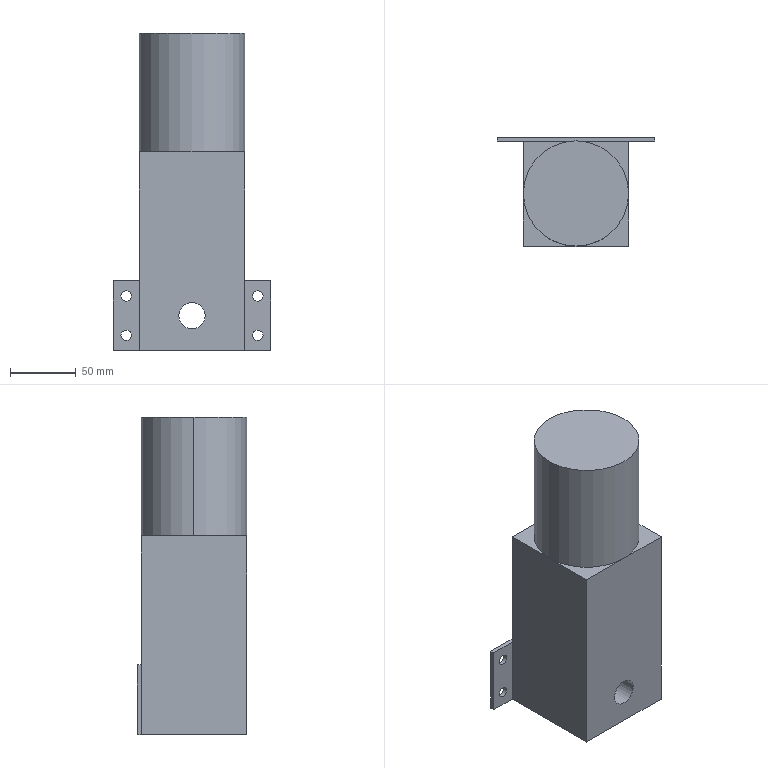Part | SolidWorks | features ICE 4, Extrusion 1 | 1 solid | 28 faces | box 120 x 83 x 241 mm | volume 1411191 mm3 | plane 16 | cylinder 12 | commonest cylinder face diameters 8 x8 20 x2 80 x2
STEP:
#1=CARTESIAN_POINT('',(0.,40.,151.));
#2=VERTEX_POINT('',#1);
#3=CARTESIAN_POINT('',(-40.,0.,151.));
#4=VERTEX_POINT('',#3);
#5=CARTESIAN_POINT('',(0.,0.,151.));
#6=DIRECTION('',(0.,0.,1.));
#7=DIRECTION('',(1.,0.,0.));
#8=AXIS2_PLACEMENT_3D('',#5,#6,#7);
#9=CIRCLE('',#8,40.);
#10=EDGE_CURVE('',#2,#4,#9,.T.);
#11=ORIENTED_EDGE('',*,*,#10,.T.);
#12=CARTESIAN_POINT('',(-40.,0.,241.));
#13=VERTEX_POINT('',#12);
#14=CARTESIAN_POINT('',(-40.,0.,151.));
#15=DIRECTION('',(0.,0.,1.));
#16=VECTOR('',#15,1000.);
#17=LINE('',#14,#16);
#18=EDGE_CURVE('',#4,#13,#17,.T.);
#19=ORIENTED_EDGE('',*,*,#18,.T.);
#20=CARTESIAN_POINT('',(40.,0.,241.));
#21=VERTEX_POINT('',#20);
#22=CARTESIAN_POINT('',(0.,0.,241.));
#23=DIRECTION('',(0.,0.,-1.));
#24=DIRECTION('',(-1.,0.,0.));
#25=AXIS2_PLACEMENT_3D('',#22,#23,#24);
#26=CIRCLE('',#25,40.);
#27=EDGE_CURVE('',#13,#21,#26,.T.);
#28=ORIENTED_EDGE('',*,*,#27,.T.);
#29=CARTESIAN_POINT('',(40.,0.,151.));
#30=VERTEX_POINT('',#29);
#31=CARTESIAN_POINT('',(40.,0.,151.));
#32=DIRECTION('',(0.,0.,1.));
#33=VECTOR('',#32,1000.);
#34=LINE('',#31,#33);
#35=EDGE_CURVE('',#30,#21,#34,.T.);
#36=ORIENTED_EDGE('',*,*,#35,.F.);
#37=CARTESIAN_POINT('',(0.,0.,151.));
#38=DIRECTION('',(0.,0.,1.));
#39=DIRECTION('',(1.,0.,0.));
#40=AXIS2_PLACEMENT_3D('',#37,#38,#39);
#41=CIRCLE('',#40,40.);
#42=EDGE_CURVE('',#30,#2,#41,.T.);
#43=ORIENTED_EDGE('',*,*,#42,.T.);
#44=EDGE_LOOP('',(#11,#19,#28,#36,#43));
#45=FACE_OUTER_BOUND('',#44,.T.);
#46=CARTESIAN_POINT('',(0.,0.,151.));
#47=DIRECTION('',(0.,0.,1.));
#48=DIRECTION('',(1.,0.,0.));
#49=AXIS2_PLACEMENT_3D('',#46,#47,#48);
#50=CYLINDRICAL_SURFACE('',#49,40.);
#51=ADVANCED_FACE('',(#45),#50,.T.);
#52=CARTESIAN_POINT('',(10.,-40.,26.5));
#53=VERTEX_POINT('',#52);
#54=CARTESIAN_POINT('',(-10.,-40.,26.5));
#55=VERTEX_POINT('',#54);
#56=CARTESIAN_POINT('',(0.,-40.,26.5));
#57=DIRECTION('',(0.,1.,0.));
#58=DIRECTION('',(-1.,0.,0.));
#59=AXIS2_PLACEMENT_3D('',#56,#57,#58);
#60=CIRCLE('',#59,10.);
#61=EDGE_CURVE('',#53,#55,#60,.T.);
#62=ORIENTED_EDGE('',*,*,#61,.F.);
#63=CARTESIAN_POINT('',(10.,43.,26.5));
#64=VERTEX_POINT('',#63);
#65=CARTESIAN_POINT('',(10.,-40.,26.5));
#66=DIRECTION('',(0.,1.,0.));
#67=VECTOR('',#66,1000.);
#68=LINE('',#65,#67);
#69=EDGE_CURVE('',#53,#64,#68,.T.);
#70=ORIENTED_EDGE('',*,*,#69,.T.);
#71=CARTESIAN_POINT('',(-10.,43.,26.5));
#72=VERTEX_POINT('',#71);
#73=CARTESIAN_POINT('',(0.,43.,26.5));
#74=DIRECTION('',(0.,1.,0.));
#75=DIRECTION('',(-1.,0.,0.));
#76=AXIS2_PLACEMENT_3D('',#73,#74,#75);
#77=CIRCLE('',#76,10.);
#78=EDGE_CURVE('',#64,#72,#77,.T.);
#79=ORIENTED_EDGE('',*,*,#78,.T.);
#80=CARTESIAN_POINT('',(-10.,-40.,26.5));
#81=DIRECTION('',(0.,1.,0.));
#82=VECTOR('',#81,1000.);
#83=LINE('',#80,#82);
#84=EDGE_CURVE('',#55,#72,#83,.T.);
#85=ORIENTED_EDGE('',*,*,#84,.F.);
#86=EDGE_LOOP('',(#62,#70,#79,#85));
#87=FACE_OUTER_BOUND('',#86,.T.);
#88=CARTESIAN_POINT('',(0.,-40.,26.5));
#89=DIRECTION('',(0.,1.,0.));
#90=DIRECTION('',(-1.,0.,0.));
#91=AXIS2_PLACEMENT_3D('',#88,#89,#90);
#92=CYLINDRICAL_SURFACE('',#91,10.);
#93=ADVANCED_FACE('',(#87),#92,.F.);
#94=CARTESIAN_POINT('',(-46.,40.,41.5));
#95=VERTEX_POINT('',#94);
#96=CARTESIAN_POINT('',(-54.,40.,41.5));
#97=VERTEX_POINT('',#96);
#98=CARTESIAN_POINT('',(-50.,40.,41.5));
#99=DIRECTION('',(0.,1.,0.));
#100=DIRECTION('',(-1.,0.,0.));
#101=AXIS2_PLACEMENT_3D('',#98,#99,#100);
#102=CIRCLE('',#101,4.);
#103=EDGE_CURVE('',#95,#97,#102,.T.);
#104=ORIENTED_EDGE('',*,*,#103,.F.);
#105=CARTESIAN_POINT('',(-46.,43.,41.5));
#106=VERTEX_POINT('',#105);
#107=CARTESIAN_POINT('',(-46.,-40.,41.5));
#108=DIRECTION('',(0.,1.,0.));
#109=VECTOR('',#108,1000.);
#110=LINE('',#107,#109);
#111=EDGE_CURVE('',#95,#106,#110,.T.);
#112=ORIENTED_EDGE('',*,*,#111,.T.);
#113=CARTESIAN_POINT('',(-54.,43.,41.5));
#114=VERTEX_POINT('',#113);
#115=CARTESIAN_POINT('',(-50.,43.,41.5));
#116=DIRECTION('',(0.,1.,0.));
#117=DIRECTION('',(-1.,0.,0.));
#118=AXIS2_PLACEMENT_3D('',#115,#116,#117);
#119=CIRCLE('',#118,4.);
#120=EDGE_CURVE('',#106,#114,#119,.T.);
#121=ORIENTED_EDGE('',*,*,#120,.T.);
#122=CARTESIAN_POINT('',(-54.,-40.,41.5));
#123=DIRECTION('',(0.,1.,0.));
#124=VECTOR('',#123,1000.);
#125=LINE('',#122,#124);
#126=EDGE_CURVE('',#97,#114,#125,.T.);
#127=ORIENTED_EDGE('',*,*,#126,.F.);
#128=EDGE_LOOP('',(#104,#112,#121,#127));
#129=FACE_OUTER_BOUND('',#128,.T.);
#130=CARTESIAN_POINT('',(-50.,-40.,41.5));
#131=DIRECTION('',(0.,1.,0.));
#132=DIRECTION('',(-1.,0.,0.));
#133=AXIS2_PLACEMENT_3D('',#130,#131,#132);
#134=CYLINDRICAL_SURFACE('',#133,4.);
#135=ADVANCED_FACE('',(#129),#134,.F.);
#136=CARTESIAN_POINT('',(54.,40.,41.5));
#137=VERTEX_POINT('',#136);
#138=CARTESIAN_POINT('',(46.,40.,41.5));
#139=VERTEX_POINT('',#138);
#140=CARTESIAN_POINT('',(50.,40.,41.5));
#141=DIRECTION('',(0.,1.,0.));
#142=DIRECTION('',(-1.,0.,0.));
#143=AXIS2_PLACEMENT_3D('',#140,#141,#142);
#144=CIRCLE('',#143,4.);
#145=EDGE_CURVE('',#137,#139,#144,.T.);
#146=ORIENTED_EDGE('',*,*,#145,.F.);
#147=CARTESIAN_POINT('',(54.,43.,41.5));
#148=VERTEX_POINT('',#147);
#149=CARTESIAN_POINT('',(54.,-40.,41.5));
#150=DIRECTION('',(0.,1.,0.));
#151=VECTOR('',#150,1000.);
#152=LINE('',#149,#151);
#153=EDGE_CURVE('',#137,#148,#152,.T.);
#154=ORIENTED_EDGE('',*,*,#153,.T.);
#155=CARTESIAN_POINT('',(46.,43.,41.5));
#156=VERTEX_POINT('',#155);
#157=CARTESIAN_POINT('',(50.,43.,41.5));
#158=DIRECTION('',(0.,1.,0.));
#159=DIRECTION('',(-1.,0.,0.));
#160=AXIS2_PLACEMENT_3D('',#157,#158,#159);
#161=CIRCLE('',#160,4.);
#162=EDGE_CURVE('',#148,#156,#161,.T.);
#163=ORIENTED_EDGE('',*,*,#162,.T.);
#164=CARTESIAN_POINT('',(46.,-40.,41.5));
#165=DIRECTION('',(0.,1.,0.));
#166=VECTOR('',#165,1000.);
#167=LINE('',#164,#166);
#168=EDGE_CURVE('',#139,#156,#167,.T.);
#169=ORIENTED_EDGE('',*,*,#168,.F.);
#170=EDGE_LOOP('',(#146,#154,#163,#169));
#171=FACE_OUTER_BOUND('',#170,.T.);
#172=CARTESIAN_POINT('',(50.,-40.,41.5));
#173=DIRECTION('',(0.,1.,0.));
#174=DIRECTION('',(-1.,0.,0.));
#175=AXIS2_PLACEMENT_3D('',#172,#173,#174);
#176=CYLINDRICAL_SURFACE('',#175,4.);
#177=ADVANCED_FACE('',(#171),#176,.F.);
#178=CARTESIAN_POINT('',(54.,40.,11.5));
#179=VERTEX_POINT('',#178);
#180=CARTESIAN_POINT('',(46.,40.,11.5));
#181=VERTEX_POINT('',#180);
#182=CARTESIAN_POINT('',(50.,40.,11.5));
#183=DIRECTION('',(0.,1.,0.));
#184=DIRECTION('',(-1.,0.,0.));
#185=AXIS2_PLACEMENT_3D('',#182,#183,#184);
#186=CIRCLE('',#185,4.);
#187=EDGE_CURVE('',#179,#181,#186,.T.);
#188=ORIENTED_EDGE('',*,*,#187,.F.);
#189=CARTESIAN_POINT('',(54.,43.,11.5));
#190=VERTEX_POINT('',#189);
#191=CARTESIAN_POINT('',(54.,-40.,11.5));
#192=DIRECTION('',(0.,1.,0.));
#193=VECTOR('',#192,1000.);
#194=LINE('',#191,#193);
#195=EDGE_CURVE('',#179,#190,#194,.T.);
#196=ORIENTED_EDGE('',*,*,#195,.T.);
#197=CARTESIAN_POINT('',(46.,43.,11.5));
#198=VERTEX_POINT('',#197);
#199=CARTESIAN_POINT('',(50.,43.,11.5));
#200=DIRECTION('',(0.,1.,0.));
#201=DIRECTION('',(-1.,0.,0.));
#202=AXIS2_PLACEMENT_3D('',#199,#200,#201);
#203=CIRCLE('',#202,4.);
#204=EDGE_CURVE('',#190,#198,#203,.T.);
#205=ORIENTED_EDGE('',*,*,#204,.T.);
#206=CARTESIAN_POINT('',(46.,-40.,11.5));
#207=DIRECTION('',(0.,1.,0.));
#208=VECTOR('',#207,1000.);
#209=LINE('',#206,#208);
#210=EDGE_CURVE('',#181,#198,#209,.T.);
#211=ORIENTED_EDGE('',*,*,#210,.F.);
#212=EDGE_LOOP('',(#188,#196,#205,#211));
#213=FACE_OUTER_BOUND('',#212,.T.);
#214=CARTESIAN_POINT('',(50.,-40.,11.5));
#215=DIRECTION('',(0.,1.,0.));
#216=DIRECTION('',(-1.,0.,0.));
#217=AXIS2_PLACEMENT_3D('',#214,#215,#216);
#218=CYLINDRICAL_SURFACE('',#217,4.);
#219=ADVANCED_FACE('',(#213),#218,.F.);
#220=CARTESIAN_POINT('',(-46.,40.,11.5));
#221=VERTEX_POINT('',#220);
#222=CARTESIAN_POINT('',(-54.,40.,11.5));
#223=VERTEX_POINT('',#222);
#224=CARTESIAN_POINT('',(-50.,40.,11.5));
#225=DIRECTION('',(0.,1.,0.));
#226=DIRECTION('',(-1.,0.,0.));
#227=AXIS2_PLACEMENT_3D('',#224,#225,#226);
#228=CIRCLE('',#227,4.);
#229=EDGE_CURVE('',#221,#223,#228,.T.);
#230=ORIENTED_EDGE('',*,*,#229,.F.);
#231=CARTESIAN_POINT('',(-46.,43.,11.5));
#232=VERTEX_POINT('',#231);
#233=CARTESIAN_POINT('',(-46.,-40.,11.5));
#234=DIRECTION('',(0.,1.,0.));
#235=VECTOR('',#234,1000.);
#236=LINE('',#233,#235);
#237=EDGE_CURVE('',#221,#232,#236,.T.);
#238=ORIENTED_EDGE('',*,*,#237,.T.);
#239=CARTESIAN_POINT('',(-54.,43.,11.5));
#240=VERTEX_POINT('',#239);
#241=CARTESIAN_POINT('',(-50.,43.,11.5));
#242=DIRECTION('',(0.,1.,0.));
#243=DIRECTION('',(-1.,0.,0.));
#244=AXIS2_PLACEMENT_3D('',#241,#242,#243);
#245=CIRCLE('',#244,4.);
#246=EDGE_CURVE('',#232,#240,#245,.T.);
#247=ORIENTED_EDGE('',*,*,#246,.T.);
#248=CARTESIAN_POINT('',(-54.,-40.,11.5));
#249=DIRECTION('',(0.,1.,0.));
#250=VECTOR('',#249,1000.);
#251=LINE('',#248,#250);
#252=EDGE_CURVE('',#223,#240,#251,.T.);
#253=ORIENTED_EDGE('',*,*,#252,.F.);
#254=EDGE_LOOP('',(#230,#238,#247,#253));
#255=FACE_OUTER_BOUND('',#254,.T.);
#256=CARTESIAN_POINT('',(-50.,-40.,11.5));
#257=DIRECTION('',(0.,1.,0.));
#258=DIRECTION('',(-1.,0.,0.));
#259=AXIS2_PLACEMENT_3D('',#256,#257,#258);
#260=CYLINDRICAL_SURFACE('',#259,4.);
#261=ADVANCED_FACE('',(#255),#260,.F.);
#262=CARTESIAN_POINT('',(40.,40.,151.));
#263=VERTEX_POINT('',#262);
#264=CARTESIAN_POINT('',(40.,40.,151.));
#265=DIRECTION('',(-1.,0.,0.));
#266=VECTOR('',#265,1000.);
#267=LINE('',#264,#266);
#268=EDGE_CURVE('',#263,#2,#267,.T.);
#269=ORIENTED_EDGE('',*,*,#268,.F.);
#270=CARTESIAN_POINT('',(40.,40.,53.));
#271=VERTEX_POINT('',#270);
#272=CARTESIAN_POINT('',(40.,40.,241.));
#273=DIRECTION('',(0.,0.,-1.));
#274=VECTOR('',#273,1000.);
#275=LINE('',#272,#274);
#276=EDGE_CURVE('',#263,#271,#275,.T.);
#277=ORIENTED_EDGE('',*,*,#276,.T.);
#278=CARTESIAN_POINT('',(-40.,40.,53.));
#279=VERTEX_POINT('',#278);
#280=CARTESIAN_POINT('',(-60.,40.,53.));
#281=DIRECTION('',(1.,0.,0.));
#282=VECTOR('',#281,1000.);
#283=LINE('',#280,#282);
#284=EDGE_CURVE('',#279,#271,#283,.T.);
#285=ORIENTED_EDGE('',*,*,#284,.F.);
#286=CARTESIAN_POINT('',(-40.,40.,151.));
#287=VERTEX_POINT('',#286);
#288=CARTESIAN_POINT('',(-40.,40.,241.));
#289=DIRECTION('',(0.,0.,-1.));
#290=VECTOR('',#289,1000.);
#291=LINE('',#288,#290);
#292=EDGE_CURVE('',#287,#279,#291,.T.);
#293=ORIENTED_EDGE('',*,*,#292,.F.);
#294=CARTESIAN_POINT('',(40.,40.,151.));
#295=DIRECTION('',(-1.,0.,0.));
#296=VECTOR('',#295,1000.);
#297=LINE('',#294,#296);
#298=EDGE_CURVE('',#2,#287,#297,.T.);
#299=ORIENTED_EDGE('',*,*,#298,.F.);
#300=EDGE_LOOP('',(#269,#277,#285,#293,#299));
#301=FACE_OUTER_BOUND('',#300,.T.);
#302=CARTESIAN_POINT('',(40.,40.,241.));
#303=DIRECTION('',(0.,-1.,0.));
#304=DIRECTION('',(1.,0.,0.));
#305=AXIS2_PLACEMENT_3D('',#302,#303,#304);
#306=PLANE('',#305);
#307=ADVANCED_FACE('',(#301),#306,.F.);
#308=CARTESIAN_POINT('',(-40.,40.,151.));
#309=DIRECTION('',(0.,-1.,0.));
#310=VECTOR('',#309,1000.);
#311=LINE('',#308,#310);
#312=EDGE_CURVE('',#287,#4,#311,.T.);
#313=ORIENTED_EDGE('',*,*,#312,.F.);
#314=ORIENTED_EDGE('',*,*,#292,.T.);
#315=CARTESIAN_POINT('',(-40.,40.,0.));
#316=VERTEX_POINT('',#315);
#317=CARTESIAN_POINT('',(-40.,40.,241.));
#318=DIRECTION('',(0.,0.,-1.));
#319=VECTOR('',#318,1000.);
#320=LINE('',#317,#319);
#321=EDGE_CURVE('',#279,#316,#320,.T.);
#322=ORIENTED_EDGE('',*,*,#321,.T.);
#323=CARTESIAN_POINT('',(-40.,-40.,0.));
#324=VERTEX_POINT('',#323);
#325=CARTESIAN_POINT('',(-40.,40.,0.));
#326=DIRECTION('',(0.,-1.,0.));
#327=VECTOR('',#326,1000.);
#328=LINE('',#325,#327);
#329=EDGE_CURVE('',#316,#324,#328,.T.);
#330=ORIENTED_EDGE('',*,*,#329,.T.);
#331=CARTESIAN_POINT('',(-40.,-40.,151.));
#332=VERTEX_POINT('',#331);
#333=CARTESIAN_POINT('',(-40.,-40.,241.));
#334=DIRECTION('',(0.,0.,-1.));
#335=VECTOR('',#334,1000.);
#336=LINE('',#333,#335);
#337=EDGE_CURVE('',#332,#324,#336,.T.);
#338=ORIENTED_EDGE('',*,*,#337,.F.);
#339=CARTESIAN_POINT('',(-40.,40.,151.));
#340=DIRECTION('',(0.,-1.,0.));
#341=VECTOR('',#340,1000.);
#342=LINE('',#339,#341);
#343=EDGE_CURVE('',#4,#332,#342,.T.);
#344=ORIENTED_EDGE('',*,*,#343,.F.);
#345=EDGE_LOOP('',(#313,#314,#322,#330,#338,#344));
#346=FACE_OUTER_BOUND('',#345,.T.);
#347=CARTESIAN_POINT('',(-40.,40.,241.));
#348=DIRECTION('',(1.,0.,0.));
#349=DIRECTION('',(0.,1.,0.));
#350=AXIS2_PLACEMENT_3D('',#347,#348,#349);
#351=PLANE('',#350);
#352=ADVANCED_FACE('',(#346),#351,.F.);
#353=CARTESIAN_POINT('',(0.,-40.,26.5));
#354=DIRECTION('',(0.,1.,0.));
#355=DIRECTION('',(-1.,0.,0.));
#356=AXIS2_PLACEMENT_3D('',#353,#354,#355);
#357=CIRCLE('',#356,10.);
#358=EDGE_CURVE('',#55,#53,#357,.T.);
#359=ORIENTED_EDGE('',*,*,#358,.T.);
#360=ORIENTED_EDGE('',*,*,#61,.T.);
#361=EDGE_LOOP('',(#359,#360));
#362=FACE_BOUND('',#361,.T.);
#363=CARTESIAN_POINT('',(0.,-40.,151.));
#364=VERTEX_POINT('',#363);
#365=CARTESIAN_POINT('',(40.,-40.,151.));
#366=DIRECTION('',(1.,0.,0.));
#367=VECTOR('',#366,1000.);
#368=LINE('',#365,#367);
#369=EDGE_CURVE('',#332,#364,#368,.T.);
#370=ORIENTED_EDGE('',*,*,#369,.F.);
#371=ORIENTED_EDGE('',*,*,#337,.T.);
#372=CARTESIAN_POINT('',(40.,-40.,0.));
#373=VERTEX_POINT('',#372);
#374=CARTESIAN_POINT('',(40.,-40.,0.));
#375=DIRECTION('',(1.,0.,0.));
#376=VECTOR('',#375,1000.);
#377=LINE('',#374,#376);
#378=EDGE_CURVE('',#324,#373,#377,.T.);
#379=ORIENTED_EDGE('',*,*,#378,.T.);
#380=CARTESIAN_POINT('',(40.,-40.,151.));
#381=VERTEX_POINT('',#380);
#382=CARTESIAN_POINT('',(40.,-40.,241.));
#383=DIRECTION('',(0.,0.,-1.));
#384=VECTOR('',#383,1000.);
#385=LINE('',#382,#384);
#386=EDGE_CURVE('',#381,#373,#385,.T.);
#387=ORIENTED_EDGE('',*,*,#386,.F.);
#388=CARTESIAN_POINT('',(40.,-40.,151.));
#389=DIRECTION('',(1.,0.,0.));
#390=VECTOR('',#389,1000.);
#391=LINE('',#388,#390);
#392=EDGE_CURVE('',#364,#381,#391,.T.);
#393=ORIENTED_EDGE('',*,*,#392,.F.);
#394=EDGE_LOOP('',(#370,#371,#379,#387,#393));
#395=FACE_OUTER_BOUND('',#394,.T.);
#396=CARTESIAN_POINT('',(40.,-40.,241.));
#397=DIRECTION('',(0.,1.,0.));
#398=DIRECTION('',(-1.,0.,0.));
#399=AXIS2_PLACEMENT_3D('',#396,#397,#398);
#400=PLANE('',#399);
#401=ADVANCED_FACE('',(#362,#395),#400,.F.);
#402=CARTESIAN_POINT('',(40.,40.,151.));
#403=DIRECTION('',(0.,1.,0.));
#404=VECTOR('',#403,1000.);
#405=LINE('',#402,#404);
#406=EDGE_CURVE('',#381,#30,#405,.T.);
#407=ORIENTED_EDGE('',*,*,#406,.F.);
#408=ORIENTED_EDGE('',*,*,#386,.T.);
#409=CARTESIAN_POINT('',(40.,40.,0.));
#410=VERTEX_POINT('',#409);
#411=CARTESIAN_POINT('',(40.,40.,0.));
#412=DIRECTION('',(0.,1.,0.));
#413=VECTOR('',#412,1000.);
#414=LINE('',#411,#413);
#415=EDGE_CURVE('',#373,#410,#414,.T.);
#416=ORIENTED_EDGE('',*,*,#415,.T.);
#417=CARTESIAN_POINT('',(40.,40.,241.));
#418=DIRECTION('',(0.,0.,-1.));
#419=VECTOR('',#418,1000.);
#420=LINE('',#417,#419);
#421=EDGE_CURVE('',#271,#410,#420,.T.);
#422=ORIENTED_EDGE('',*,*,#421,.F.);
#423=ORIENTED_EDGE('',*,*,#276,.F.);
#424=CARTESIAN_POINT('',(40.,40.,151.));
#425=DIRECTION('',(0.,1.,0.));
#426=VECTOR('',#425,1000.);
#427=LINE('',#424,#426);
#428=EDGE_CURVE('',#30,#263,#427,.T.);
#429=ORIENTED_EDGE('',*,*,#428,.F.);
#430=EDGE_LOOP('',(#407,#408,#416,#422,#423,#429));
#431=FACE_OUTER_BOUND('',#430,.T.);
#432=CARTESIAN_POINT('',(40.,40.,241.));
#433=DIRECTION('',(-1.,0.,0.));
#434=DIRECTION('',(0.,-1.,0.));
#435=AXIS2_PLACEMENT_3D('',#432,#433,#434);
#436=PLANE('',#435);
#437=ADVANCED_FACE('',(#431),#436,.F.);
#438=ORIENTED_EDGE('',*,*,#329,.F.);
#439=CARTESIAN_POINT('',(-60.,40.,0.));
#440=VERTEX_POINT('',#439);
#441=CARTESIAN_POINT('',(-60.,40.,0.));
#442=DIRECTION('',(-1.,0.,0.));
#443=VECTOR('',#442,1000.);
#444=LINE('',#441,#443);
#445=EDGE_CURVE('',#316,#440,#444,.T.);
#446=ORIENTED_EDGE('',*,*,#445,.T.);
#447=CARTESIAN_POINT('',(-60.,43.,0.));
#448=VERTEX_POINT('',#447);
#449=CARTESIAN_POINT('',(-60.,43.,0.));
#450=DIRECTION('',(0.,-1.,0.));
#451=VECTOR('',#450,1000.);
#452=LINE('',#449,#451);
#453=EDGE_CURVE('',#448,#440,#452,.T.);
#454=ORIENTED_EDGE('',*,*,#453,.F.);
#455=CARTESIAN_POINT('',(60.,43.,0.));
#456=VERTEX_POINT('',#455);
#457=CARTESIAN_POINT('',(-60.,43.,0.));
#458=DIRECTION('',(-1.,0.,0.));
#459=VECTOR('',#458,1000.);
#460=LINE('',#457,#459);
#461=EDGE_CURVE('',#456,#448,#460,.T.);
#462=ORIENTED_EDGE('',*,*,#461,.F.);
#463=CARTESIAN_POINT('',(60.,40.,0.));
#464=VERTEX_POINT('',#463);
#465=CARTESIAN_POINT('',(60.,43.,0.));
#466=DIRECTION('',(0.,-1.,0.));
#467=VECTOR('',#466,1000.);
#468=LINE('',#465,#467);
#469=EDGE_CURVE('',#456,#464,#468,.T.);
#470=ORIENTED_EDGE('',*,*,#469,.T.);
#471=CARTESIAN_POINT('',(-60.,40.,0.));
#472=DIRECTION('',(-1.,0.,0.));
#473=VECTOR('',#472,1000.);
#474=LINE('',#471,#473);
#475=EDGE_CURVE('',#464,#410,#474,.T.);
#476=ORIENTED_EDGE('',*,*,#475,.T.);
#477=ORIENTED_EDGE('',*,*,#415,.F.);
#478=ORIENTED_EDGE('',*,*,#378,.F.);
#479=EDGE_LOOP('',(#438,#446,#454,#462,#470,#476,#477,#478));
#480=FACE_OUTER_BOUND('',#479,.T.);
#481=CARTESIAN_POINT('',(0.,0.,0.));
#482=DIRECTION('',(0.,0.,-1.));
#483=DIRECTION('',(-1.,0.,0.));
#484=AXIS2_PLACEMENT_3D('',#481,#482,#483);
#485=PLANE('',#484);
#486=ADVANCED_FACE('',(#480),#485,.T.);
#487=CARTESIAN_POINT('',(50.,40.,41.5));
#488=DIRECTION('',(0.,1.,0.));
#489=DIRECTION('',(-1.,0.,0.));
#490=AXIS2_PLACEMENT_3D('',#487,#488,#489);
#491=CIRCLE('',#490,4.);
#492=EDGE_CURVE('',#139,#137,#491,.T.);
#493=ORIENTED_EDGE('',*,*,#492,.T.);
#494=ORIENTED_EDGE('',*,*,#145,.T.);
#495=EDGE_LOOP('',(#493,#494));
#496=FACE_BOUND('',#495,.T.);
#497=CARTESIAN_POINT('',(50.,40.,11.5));
#498=DIRECTION('',(0.,1.,0.));
#499=DIRECTION('',(-1.,0.,0.));
#500=AXIS2_PLACEMENT_3D('',#497,#498,#499);
#501=CIRCLE('',#500,4.);
#502=EDGE_CURVE('',#181,#179,#501,.T.);
#503=ORIENTED_EDGE('',*,*,#502,.T.);
#504=ORIENTED_EDGE('',*,*,#187,.T.);
#505=EDGE_LOOP('',(#503,#504));
#506=FACE_BOUND('',#505,.T.);
#507=CARTESIAN_POINT('',(60.,40.,53.));
#508=VERTEX_POINT('',#507);
#509=CARTESIAN_POINT('',(-60.,40.,53.));
#510=DIRECTION('',(1.,0.,0.));
#511=VECTOR('',#510,1000.);
#512=LINE('',#509,#511);
#513=EDGE_CURVE('',#271,#508,#512,.T.);
#514=ORIENTED_EDGE('',*,*,#513,.F.);
#515=ORIENTED_EDGE('',*,*,#421,.T.);
#516=ORIENTED_EDGE('',*,*,#475,.F.);
#517=CARTESIAN_POINT('',(60.,40.,0.));
#518=DIRECTION('',(0.,0.,-1.));
#519=VECTOR('',#518,1000.);
#520=LINE('',#517,#519);
#521=EDGE_CURVE('',#508,#464,#520,.T.);
#522=ORIENTED_EDGE('',*,*,#521,.F.);
#523=EDGE_LOOP('',(#514,#515,#516,#522));
#524=FACE_OUTER_BOUND('',#523,.T.);
#525=CARTESIAN_POINT('',(0.,40.,0.));
#526=DIRECTION('',(0.,1.,0.));
#527=DIRECTION('',(-1.,0.,0.));
#528=AXIS2_PLACEMENT_3D('',#525,#526,#527);
#529=PLANE('',#528);
#530=ADVANCED_FACE('',(#496,#506,#524),#529,.F.);
#531=CARTESIAN_POINT('',(-60.,40.,53.));
#532=VERTEX_POINT('',#531);
#533=CARTESIAN_POINT('',(-60.,40.,0.));
#534=DIRECTION('',(0.,0.,1.));
#535=VECTOR('',#534,1000.);
#536=LINE('',#533,#535);
#537=EDGE_CURVE('',#440,#532,#536,.T.);
#538=ORIENTED_EDGE('',*,*,#537,.T.);
#539=CARTESIAN_POINT('',(-60.,43.,53.));
#540=VERTEX_POINT('',#539);
#541=CARTESIAN_POINT('',(-60.,43.,53.));
#542=DIRECTION('',(0.,-1.,0.));
#543=VECTOR('',#542,1000.);
#544=LINE('',#541,#543);
#545=EDGE_CURVE('',#540,#532,#544,.T.);
#546=ORIENTED_EDGE('',*,*,#545,.F.);
#547=CARTESIAN_POINT('',(-60.,43.,0.));
#548=DIRECTION('',(0.,0.,1.));
#549=VECTOR('',#548,1000.);
#550=LINE('',#547,#549);
#551=EDGE_CURVE('',#448,#540,#550,.T.);
#552=ORIENTED_EDGE('',*,*,#551,.F.);
#553=ORIENTED_EDGE('',*,*,#453,.T.);
#554=EDGE_LOOP('',(#538,#546,#552,#553));
#555=FACE_OUTER_BOUND('',#554,.T.);
#556=CARTESIAN_POINT('',(-60.,43.,0.));
#557=DIRECTION('',(1.,0.,0.));
#558=DIRECTION('',(0.,0.,-1.));
#559=AXIS2_PLACEMENT_3D('',#556,#557,#558);
#560=PLANE('',#559);
#561=ADVANCED_FACE('',(#555),#560,.F.);
#562=CARTESIAN_POINT('',(-60.,40.,53.));
#563=DIRECTION('',(1.,0.,0.));
#564=VECTOR('',#563,1000.);
#565=LINE('',#562,#564);
#566=EDGE_CURVE('',#532,#279,#565,.T.);
#567=ORIENTED_EDGE('',*,*,#566,.T.);
#568=ORIENTED_EDGE('',*,*,#284,.T.);
#569=ORIENTED_EDGE('',*,*,#513,.T.);
#570=CARTESIAN_POINT('',(60.,43.,53.));
#571=VERTEX_POINT('',#570);
#572=CARTESIAN_POINT('',(60.,43.,53.));
#573=DIRECTION('',(0.,-1.,0.));
#574=VECTOR('',#573,1000.);
#575=LINE('',#572,#574);
#576=EDGE_CURVE('',#571,#508,#575,.T.);
#577=ORIENTED_EDGE('',*,*,#576,.F.);
#578=CARTESIAN_POINT('',(-60.,43.,53.));
#579=DIRECTION('',(1.,0.,0.));
#580=VECTOR('',#579,1000.);
#581=LINE('',#578,#580);
#582=EDGE_CURVE('',#540,#571,#581,.T.);
#583=ORIENTED_EDGE('',*,*,#582,.F.);
#584=ORIENTED_EDGE('',*,*,#545,.T.);
#585=EDGE_LOOP('',(#567,#568,#569,#577,#583,#584));
#586=FACE_OUTER_BOUND('',#585,.T.);
#587=CARTESIAN_POINT('',(-60.,43.,53.));
#588=DIRECTION('',(0.,0.,-1.));
#589=DIRECTION('',(-1.,0.,0.));
#590=AXIS2_PLACEMENT_3D('',#587,#588,#589);
#591=PLANE('',#590);
#592=ADVANCED_FACE('',(#586),#591,.F.);
#593=ORIENTED_EDGE('',*,*,#521,.T.);
#594=ORIENTED_EDGE('',*,*,#469,.F.);
#595=CARTESIAN_POINT('',(60.,43.,0.));
#596=DIRECTION('',(0.,0.,-1.));
#597=VECTOR('',#596,1000.);
#598=LINE('',#595,#597);
#599=EDGE_CURVE('',#571,#456,#598,.T.);
#600=ORIENTED_EDGE('',*,*,#599,.F.);
#601=ORIENTED_EDGE('',*,*,#576,.T.);
#602=EDGE_LOOP('',(#593,#594,#600,#601));
#603=FACE_OUTER_BOUND('',#602,.T.);
#604=CARTESIAN_POINT('',(60.,43.,0.));
#605=DIRECTION('',(-1.,0.,0.));
#606=DIRECTION('',(0.,-1.,0.));
#607=AXIS2_PLACEMENT_3D('',#604,#605,#606);
#608=PLANE('',#607);
#609=ADVANCED_FACE('',(#603),#608,.F.);
#610=CARTESIAN_POINT('',(0.,43.,26.5));
#611=DIRECTION('',(0.,1.,0.));
#612=DIRECTION('',(-1.,0.,0.));
#613=AXIS2_PLACEMENT_3D('',#610,#611,#612);
#614=CIRCLE('',#613,10.);
#615=EDGE_CURVE('',#72,#64,#614,.T.);
#616=ORIENTED_EDGE('',*,*,#615,.F.);
#617=ORIENTED_EDGE('',*,*,#78,.F.);
#618=EDGE_LOOP('',(#616,#617));
#619=FACE_BOUND('',#618,.T.);
#620=CARTESIAN_POINT('',(-50.,43.,41.5));
#621=DIRECTION('',(0.,1.,0.));
#622=DIRECTION('',(-1.,0.,0.));
#623=AXIS2_PLACEMENT_3D('',#620,#621,#622);
#624=CIRCLE('',#623,4.);
#625=EDGE_CURVE('',#114,#106,#624,.T.);
#626=ORIENTED_EDGE('',*,*,#625,.F.);
#627=ORIENTED_EDGE('',*,*,#120,.F.);
#628=EDGE_LOOP('',(#626,#627));
#629=FACE_BOUND('',#628,.T.);
#630=CARTESIAN_POINT('',(50.,43.,41.5));
#631=DIRECTION('',(0.,1.,0.));
#632=DIRECTION('',(-1.,0.,0.));
#633=AXIS2_PLACEMENT_3D('',#630,#631,#632);
#634=CIRCLE('',#633,4.);
#635=EDGE_CURVE('',#156,#148,#634,.T.);
#636=ORIENTED_EDGE('',*,*,#635,.F.);
#637=ORIENTED_EDGE('',*,*,#162,.F.);
#638=EDGE_LOOP('',(#636,#637));
#639=FACE_BOUND('',#638,.T.);
#640=CARTESIAN_POINT('',(50.,43.,11.5));
#641=DIRECTION('',(0.,1.,0.));
#642=DIRECTION('',(-1.,0.,0.));
#643=AXIS2_PLACEMENT_3D('',#640,#641,#642);
#644=CIRCLE('',#643,4.);
#645=EDGE_CURVE('',#198,#190,#644,.T.);
#646=ORIENTED_EDGE('',*,*,#645,.F.);
#647=ORIENTED_EDGE('',*,*,#204,.F.);
#648=EDGE_LOOP('',(#646,#647));
#649=FACE_BOUND('',#648,.T.);
#650=CARTESIAN_POINT('',(-50.,43.,11.5));
#651=DIRECTION('',(0.,1.,0.));
#652=DIRECTION('',(-1.,0.,0.));
#653=AXIS2_PLACEMENT_3D('',#650,#651,#652);
#654=CIRCLE('',#653,4.);
#655=EDGE_CURVE('',#240,#232,#654,.T.);
#656=ORIENTED_EDGE('',*,*,#655,.F.);
#657=ORIENTED_EDGE('',*,*,#246,.F.);
#658=EDGE_LOOP('',(#656,#657));
#659=FACE_BOUND('',#658,.T.);
#660=ORIENTED_EDGE('',*,*,#551,.T.);
#661=ORIENTED_EDGE('',*,*,#582,.T.);
#662=ORIENTED_EDGE('',*,*,#599,.T.);
#663=ORIENTED_EDGE('',*,*,#461,.T.);
#664=EDGE_LOOP('',(#660,#661,#662,#663));
#665=FACE_OUTER_BOUND('',#664,.T.);
#666=CARTESIAN_POINT('',(0.,43.,0.));
#667=DIRECTION('',(0.,1.,0.));
#668=DIRECTION('',(-1.,0.,0.));
#669=AXIS2_PLACEMENT_3D('',#666,#667,#668);
#670=PLANE('',#669);
#671=ADVANCED_FACE('',(#619,#629,#639,#649,#659,#665),#670,.T.);
#672=CARTESIAN_POINT('',(-50.,40.,41.5));
#673=DIRECTION('',(0.,1.,0.));
#674=DIRECTION('',(-1.,0.,0.));
#675=AXIS2_PLACEMENT_3D('',#672,#673,#674);
#676=CIRCLE('',#675,4.);
#677=EDGE_CURVE('',#97,#95,#676,.T.);
#678=ORIENTED_EDGE('',*,*,#677,.T.);
#679=ORIENTED_EDGE('',*,*,#103,.T.);
#680=EDGE_LOOP('',(#678,#679));
#681=FACE_BOUND('',#680,.T.);
#682=CARTESIAN_POINT('',(-50.,40.,11.5));
#683=DIRECTION('',(0.,1.,0.));
#684=DIRECTION('',(-1.,0.,0.));
#685=AXIS2_PLACEMENT_3D('',#682,#683,#684);
#686=CIRCLE('',#685,4.);
#687=EDGE_CURVE('',#223,#221,#686,.T.);
#688=ORIENTED_EDGE('',*,*,#687,.T.);
#689=ORIENTED_EDGE('',*,*,#229,.T.);
#690=EDGE_LOOP('',(#688,#689));
#691=FACE_BOUND('',#690,.T.);
#692=ORIENTED_EDGE('',*,*,#321,.F.);
#693=ORIENTED_EDGE('',*,*,#566,.F.);
#694=ORIENTED_EDGE('',*,*,#537,.F.);
#695=ORIENTED_EDGE('',*,*,#445,.F.);
#696=EDGE_LOOP('',(#692,#693,#694,#695));
#697=FACE_OUTER_BOUND('',#696,.T.);
#698=CARTESIAN_POINT('',(0.,40.,0.));
#699=DIRECTION('',(0.,1.,0.));
#700=DIRECTION('',(-1.,0.,0.));
#701=AXIS2_PLACEMENT_3D('',#698,#699,#700);
#702=PLANE('',#701);
#703=ADVANCED_FACE('',(#681,#691,#697),#702,.F.);
#704=ORIENTED_EDGE('',*,*,#237,.F.);
#705=ORIENTED_EDGE('',*,*,#687,.F.);
#706=ORIENTED_EDGE('',*,*,#252,.T.);
#707=ORIENTED_EDGE('',*,*,#655,.T.);
#708=EDGE_LOOP('',(#704,#705,#706,#707));
#709=FACE_OUTER_BOUND('',#708,.T.);
#710=CARTESIAN_POINT('',(-50.,-40.,11.5));
#711=DIRECTION('',(0.,1.,0.));
#712=DIRECTION('',(-1.,0.,0.));
#713=AXIS2_PLACEMENT_3D('',#710,#711,#712);
#714=CYLINDRICAL_SURFACE('',#713,4.);
#715=ADVANCED_FACE('',(#709),#714,.F.);
#716=ORIENTED_EDGE('',*,*,#195,.F.);
#717=ORIENTED_EDGE('',*,*,#502,.F.);
#718=ORIENTED_EDGE('',*,*,#210,.T.);
#719=ORIENTED_EDGE('',*,*,#645,.T.);
#720=EDGE_LOOP('',(#716,#717,#718,#719));
#721=FACE_OUTER_BOUND('',#720,.T.);
#722=CARTESIAN_POINT('',(50.,-40.,11.5));
#723=DIRECTION('',(0.,1.,0.));
#724=DIRECTION('',(-1.,0.,0.));
#725=AXIS2_PLACEMENT_3D('',#722,#723,#724);
#726=CYLINDRICAL_SURFACE('',#725,4.);
#727=ADVANCED_FACE('',(#721),#726,.F.);
#728=ORIENTED_EDGE('',*,*,#153,.F.);
#729=ORIENTED_EDGE('',*,*,#492,.F.);
#730=ORIENTED_EDGE('',*,*,#168,.T.);
#731=ORIENTED_EDGE('',*,*,#635,.T.);
#732=EDGE_LOOP('',(#728,#729,#730,#731));
#733=FACE_OUTER_BOUND('',#732,.T.);
#734=CARTESIAN_POINT('',(50.,-40.,41.5));
#735=DIRECTION('',(0.,1.,0.));
#736=DIRECTION('',(-1.,0.,0.));
#737=AXIS2_PLACEMENT_3D('',#734,#735,#736);
#738=CYLINDRICAL_SURFACE('',#737,4.);
#739=ADVANCED_FACE('',(#733),#738,.F.);
#740=ORIENTED_EDGE('',*,*,#111,.F.);
#741=ORIENTED_EDGE('',*,*,#677,.F.);
#742=ORIENTED_EDGE('',*,*,#126,.T.);
#743=ORIENTED_EDGE('',*,*,#625,.T.);
#744=EDGE_LOOP('',(#740,#741,#742,#743));
#745=FACE_OUTER_BOUND('',#744,.T.);
#746=CARTESIAN_POINT('',(-50.,-40.,41.5));
#747=DIRECTION('',(0.,1.,0.));
#748=DIRECTION('',(-1.,0.,0.));
#749=AXIS2_PLACEMENT_3D('',#746,#747,#748);
#750=CYLINDRICAL_SURFACE('',#749,4.);
#751=ADVANCED_FACE('',(#745),#750,.F.);
#752=ORIENTED_EDGE('',*,*,#69,.F.);
#753=ORIENTED_EDGE('',*,*,#358,.F.);
#754=ORIENTED_EDGE('',*,*,#84,.T.);
#755=ORIENTED_EDGE('',*,*,#615,.T.);
#756=EDGE_LOOP('',(#752,#753,#754,#755));
#757=FACE_OUTER_BOUND('',#756,.T.);
#758=CARTESIAN_POINT('',(0.,-40.,26.5));
#759=DIRECTION('',(0.,1.,0.));
#760=DIRECTION('',(-1.,0.,0.));
#761=AXIS2_PLACEMENT_3D('',#758,#759,#760);
#762=CYLINDRICAL_SURFACE('',#761,10.);
#763=ADVANCED_FACE('',(#757),#762,.F.);
#764=ORIENTED_EDGE('',*,*,#268,.T.);
#765=ORIENTED_EDGE('',*,*,#42,.F.);
#766=ORIENTED_EDGE('',*,*,#428,.T.);
#767=EDGE_LOOP('',(#764,#765,#766));
#768=FACE_OUTER_BOUND('',#767,.T.);
#769=CARTESIAN_POINT('',(0.,1.5,151.));
#770=DIRECTION('',(0.,0.,1.));
#771=DIRECTION('',(1.,0.,0.));
#772=AXIS2_PLACEMENT_3D('',#769,#770,#771);
#773=PLANE('',#772);
#774=ADVANCED_FACE('',(#768),#773,.T.);
#775=ORIENTED_EDGE('',*,*,#298,.T.);
#776=ORIENTED_EDGE('',*,*,#312,.T.);
#777=ORIENTED_EDGE('',*,*,#10,.F.);
#778=EDGE_LOOP('',(#775,#776,#777));
#779=FACE_OUTER_BOUND('',#778,.T.);
#780=CARTESIAN_POINT('',(0.,1.5,151.));
#781=DIRECTION('',(0.,0.,1.));
#782=DIRECTION('',(1.,0.,0.));
#783=AXIS2_PLACEMENT_3D('',#780,#781,#782);
#784=PLANE('',#783);
#785=ADVANCED_FACE('',(#779),#784,.T.);
#786=ORIENTED_EDGE('',*,*,#343,.T.);
#787=ORIENTED_EDGE('',*,*,#369,.T.);
#788=CARTESIAN_POINT('',(0.,0.,151.));
#789=DIRECTION('',(0.,0.,1.));
#790=DIRECTION('',(1.,0.,0.));
#791=AXIS2_PLACEMENT_3D('',#788,#789,#790);
#792=CIRCLE('',#791,40.);
#793=EDGE_CURVE('',#4,#364,#792,.T.);
#794=ORIENTED_EDGE('',*,*,#793,.F.);
#795=EDGE_LOOP('',(#786,#787,#794));
#796=FACE_OUTER_BOUND('',#795,.T.);
#797=CARTESIAN_POINT('',(0.,1.5,151.));
#798=DIRECTION('',(0.,0.,1.));
#799=DIRECTION('',(1.,0.,0.));
#800=AXIS2_PLACEMENT_3D('',#797,#798,#799);
#801=PLANE('',#800);
#802=ADVANCED_FACE('',(#796),#801,.T.);
#803=ORIENTED_EDGE('',*,*,#392,.T.);
#804=ORIENTED_EDGE('',*,*,#406,.T.);
#805=CARTESIAN_POINT('',(0.,0.,151.));
#806=DIRECTION('',(0.,0.,1.));
#807=DIRECTION('',(1.,0.,0.));
#808=AXIS2_PLACEMENT_3D('',#805,#806,#807);
#809=CIRCLE('',#808,40.);
#810=EDGE_CURVE('',#364,#30,#809,.T.);
#811=ORIENTED_EDGE('',*,*,#810,.F.);
#812=EDGE_LOOP('',(#803,#804,#811));
#813=FACE_OUTER_BOUND('',#812,.T.);
#814=CARTESIAN_POINT('',(0.,1.5,151.));
#815=DIRECTION('',(0.,0.,1.));
#816=DIRECTION('',(1.,0.,0.));
#817=AXIS2_PLACEMENT_3D('',#814,#815,#816);
#818=PLANE('',#817);
#819=ADVANCED_FACE('',(#813),#818,.T.);
#820=ORIENTED_EDGE('',*,*,#18,.F.);
#821=ORIENTED_EDGE('',*,*,#793,.T.);
#822=ORIENTED_EDGE('',*,*,#810,.T.);
#823=ORIENTED_EDGE('',*,*,#35,.T.);
#824=CARTESIAN_POINT('',(0.,0.,241.));
#825=DIRECTION('',(0.,0.,-1.));
#826=DIRECTION('',(-1.,0.,0.));
#827=AXIS2_PLACEMENT_3D('',#824,#825,#826);
#828=CIRCLE('',#827,40.);
#829=EDGE_CURVE('',#21,#13,#828,.T.);
#830=ORIENTED_EDGE('',*,*,#829,.T.);
#831=EDGE_LOOP('',(#820,#821,#822,#823,#830));
#832=FACE_OUTER_BOUND('',#831,.T.);
#833=CARTESIAN_POINT('',(0.,0.,151.));
#834=DIRECTION('',(0.,0.,1.));
#835=DIRECTION('',(1.,0.,0.));
#836=AXIS2_PLACEMENT_3D('',#833,#834,#835);
#837=CYLINDRICAL_SURFACE('',#836,40.);
#838=ADVANCED_FACE('',(#832),#837,.T.);
#839=ORIENTED_EDGE('',*,*,#829,.F.);
#840=ORIENTED_EDGE('',*,*,#27,.F.);
#841=EDGE_LOOP('',(#839,#840));
#842=FACE_OUTER_BOUND('',#841,.T.);
#843=CARTESIAN_POINT('',(0.,0.,241.));
#844=DIRECTION('',(0.,0.,-1.));
#845=DIRECTION('',(-1.,0.,0.));
#846=AXIS2_PLACEMENT_3D('',#843,#844,#845);
#847=PLANE('',#846);
#848=ADVANCED_FACE('',(#842),#847,.F.);
#849=CLOSED_SHELL('',(#51,#93,#135,#177,#219,#261,#307,#352,#401,#437,#486,#530,#561,#592,#609,#671,#703,#715,#727,#739,#751,#763,#774,#785,#802,#819,#838,#848));
#850=MANIFOLD_SOLID_BREP('',#849);
#851=CARTESIAN_POINT('',(0.,0.,0.));
#852=DIRECTION('',(0.,0.,1.));
#853=DIRECTION('',(1.,0.,0.));
#854=AXIS2_PLACEMENT_3D('',#851,#852,#853);
#855=(LENGTH_UNIT()NAMED_UNIT(*)SI_UNIT(.MILLI.,.METRE.));
#856=UNCERTAINTY_MEASURE_WITH_UNIT(LENGTH_MEASURE(0.00001),#855,'','');
#857=(NAMED_UNIT(*)PLANE_ANGLE_UNIT()SI_UNIT($,.RADIAN.));
#858=(NAMED_UNIT(*)SI_UNIT($,.STERADIAN.)SOLID_ANGLE_UNIT());
#859=(GEOMETRIC_REPRESENTATION_CONTEXT(3)GLOBAL_UNCERTAINTY_ASSIGNED_CONTEXT((#856))GLOBAL_UNIT_ASSIGNED_CONTEXT((#855,#857,#858))REPRESENTATION_CONTEXT('',''));
#860=ADVANCED_BREP_SHAPE_REPRESENTATION('',(#850,#854),#859);